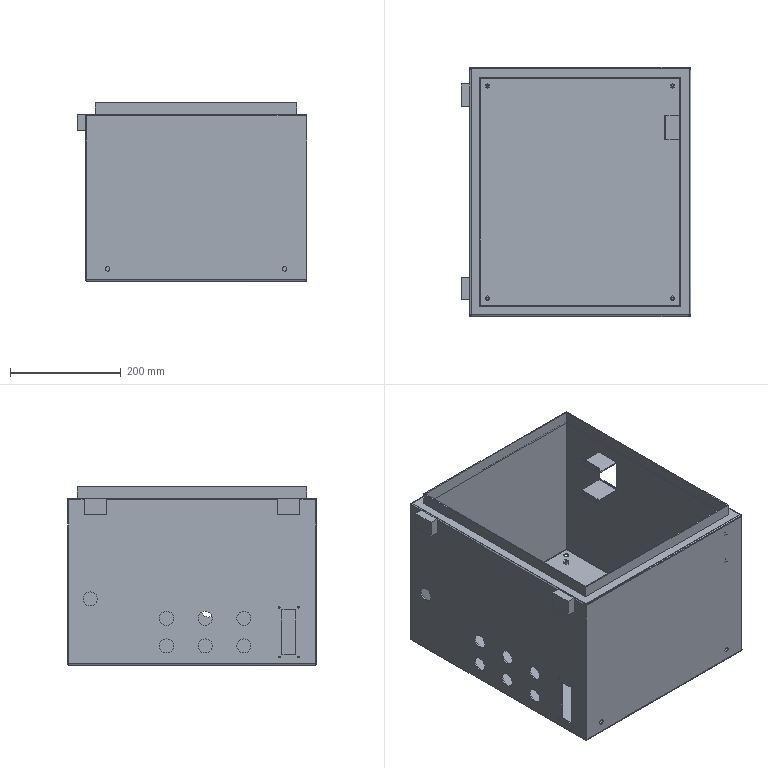Part | STEP file | Lower ctrl box 1 | 1 solid | 231 faces | box 415 x 450 x 322.745 mm | volume 1529445 mm3 | cylinder 110 | plane 97 | spline 24 | commonest cylinder face diameters 8.5 x24 3.3 x18 25.5 x16 1.473 x8 4 x8 4.5 x8